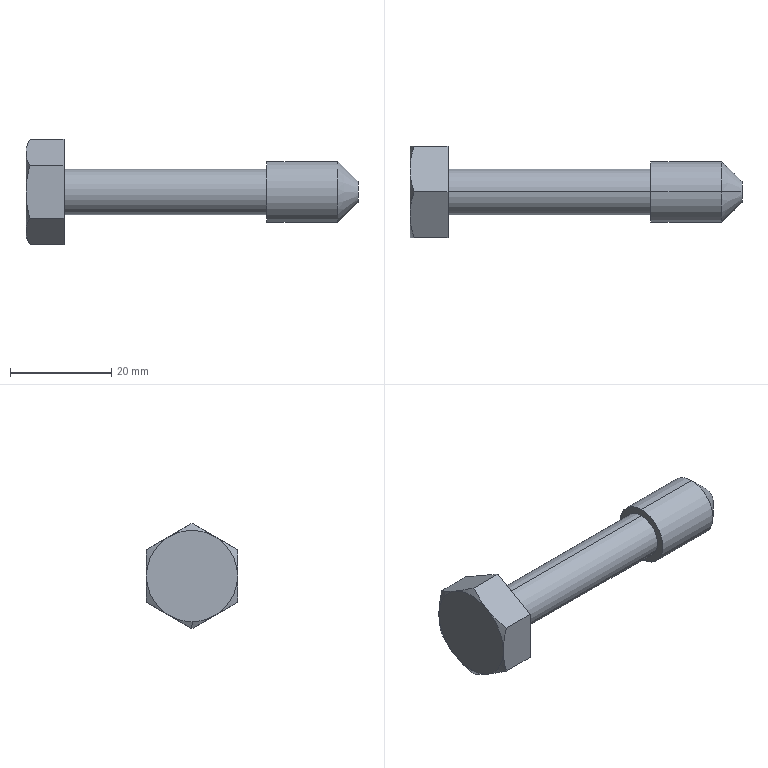Part | STEP file | hexagon screws with waisted shank gb_GB_SQUARE_AND_HEXAGON_TYPE1 M12X55-N | 1 solid | 23 faces | box 65.5 x 18 x 20.785 mm | volume 6444 mm3 | plane 10 | cone 9 | cylinder 4 | commonest cylinder face diameters 9 x2 12 x2